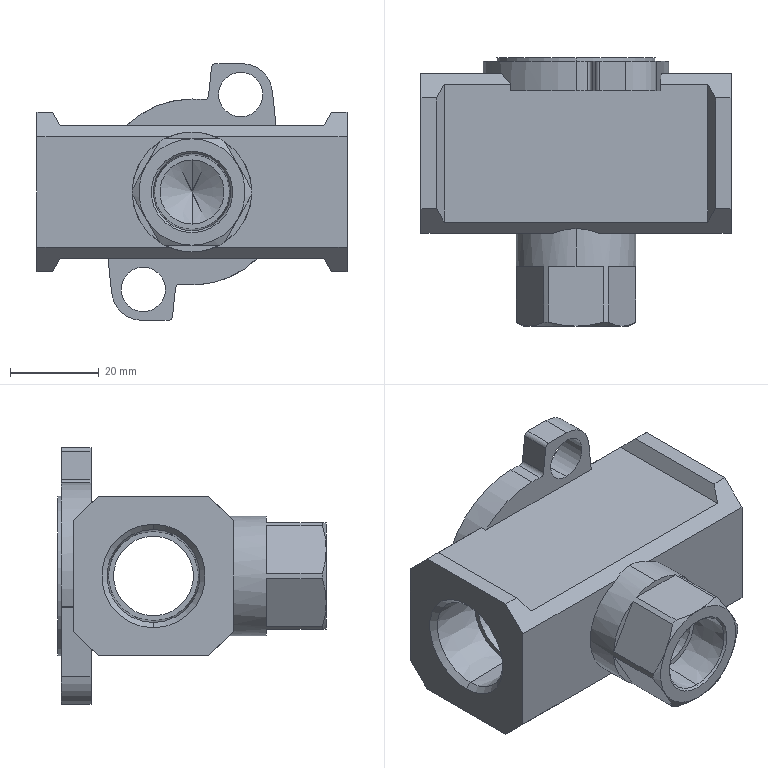Part | STEP file | AC40-04-KSTV-38JNR_AC3009A VHS Body-1 | 1 solid | 94 faces | box 70 x 60.6 x 58 mm | volume 70876 mm3 | plane 48 | cylinder 26 | cone 20 | commonest cylinder face diameters 2 x7 10 x4 18 x4 42 x3 14 x2 14.5 x2